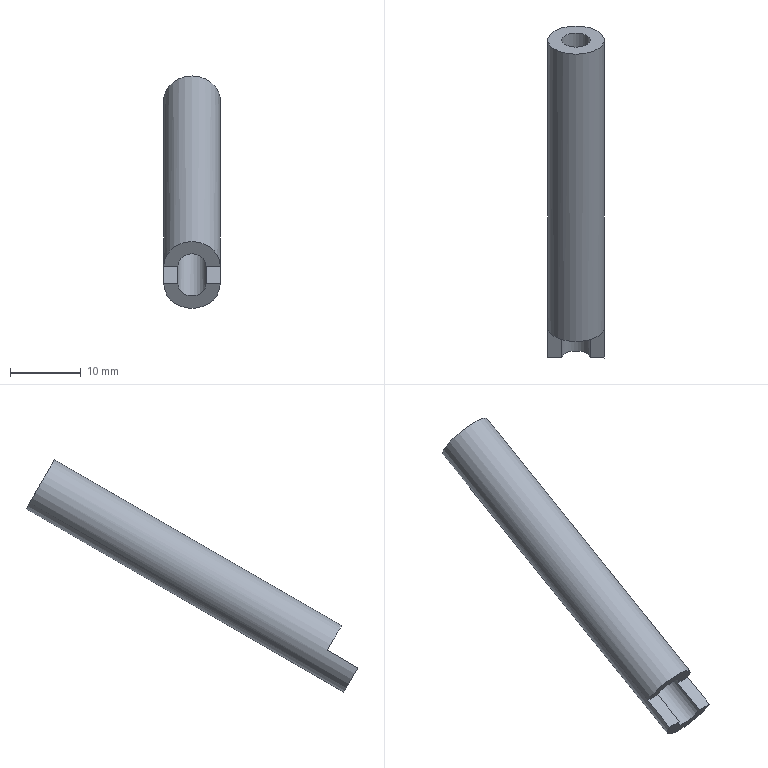Part | NX | features solid 2 | 1 solid | 7 faces | box 8 x 46.958 x 32.885 mm | volume 1862 mm3 | plane 5 | cylinder 2 | commonest cylinder face diameters 4.003 x1 8 x1
STEP:
#1=CARTESIAN_POINT('',(-144.025,135.478,18.602));
#2=VERTEX_POINT('',#1);
#3=CARTESIAN_POINT('',(-136.025,135.478,18.602));
#4=VERTEX_POINT('',#3);
#5=CARTESIAN_POINT('',(-140.025,135.478,18.602));
#6=DIRECTION('',(0.000000832,0.866,0.5));
#7=DIRECTION('',(-1.,0.,0.000001664));
#8=AXIS2_PLACEMENT_3D('',#5,#6,#7);
#9=CIRCLE('',#8,4.);
#10=EDGE_CURVE('',#2,#4,#9,.F.);
#11=ORIENTED_EDGE('',*,*,#10,.T.);
#12=CARTESIAN_POINT('',(-138.023,135.478,18.602));
#13=VERTEX_POINT('',#12);
#14=CARTESIAN_POINT('',(-145.025,135.478,18.602));
#15=DIRECTION('',(1.,0.,-0.000001664));
#16=VECTOR('',#15,1000.);
#17=LINE('',#14,#16);
#18=EDGE_CURVE('',#4,#13,#17,.F.);
#19=ORIENTED_EDGE('',*,*,#18,.T.);
#20=CARTESIAN_POINT('',(-142.026,135.478,18.602));
#21=VERTEX_POINT('',#20);
#22=CARTESIAN_POINT('',(-140.025,135.478,18.602));
#23=DIRECTION('',(0.000000832,0.866,0.5));
#24=DIRECTION('',(-1.,0.,0.000001664));
#25=AXIS2_PLACEMENT_3D('',#22,#23,#24);
#26=CIRCLE('',#25,2.002);
#27=EDGE_CURVE('',#21,#13,#26,.F.);
#28=ORIENTED_EDGE('',*,*,#27,.F.);
#29=CARTESIAN_POINT('',(-145.025,135.478,18.602));
#30=DIRECTION('',(1.,0.,-0.000001664));
#31=VECTOR('',#30,1000.);
#32=LINE('',#29,#31);
#33=EDGE_CURVE('',#21,#2,#32,.F.);
#34=ORIENTED_EDGE('',*,*,#33,.T.);
#35=EDGE_LOOP('',(#11,#19,#28,#34));
#36=FACE_BOUND('',#35,.T.);
#37=CARTESIAN_POINT('',(-140.025,135.478,18.602));
#38=DIRECTION('',(-0.000000832,-0.866,-0.5));
#39=DIRECTION('',(0.,0.5,-0.866));
#40=AXIS2_PLACEMENT_3D('',#37,#38,#39);
#41=PLANE('',#40);
#42=ADVANCED_FACE('',(#36),#41,.T.);
#43=ORIENTED_EDGE('',*,*,#10,.F.);
#44=CARTESIAN_POINT('',(-144.025,139.808,21.102));
#45=VERTEX_POINT('',#44);
#46=CARTESIAN_POINT('',(-144.025,135.478,18.602));
#47=DIRECTION('',(0.000000832,0.866,0.5));
#48=VECTOR('',#47,1000.);
#49=LINE('',#46,#48);
#50=EDGE_CURVE('',#2,#45,#49,.T.);
#51=ORIENTED_EDGE('',*,*,#50,.T.);
#52=CARTESIAN_POINT('',(-136.025,139.808,21.102));
#53=VERTEX_POINT('',#52);
#54=CARTESIAN_POINT('',(-140.025,139.808,21.102));
#55=DIRECTION('',(0.000000832,0.866,0.5));
#56=DIRECTION('',(0.,0.5,-0.866));
#57=AXIS2_PLACEMENT_3D('',#54,#55,#56);
#58=CIRCLE('',#57,4.);
#59=EDGE_CURVE('',#53,#45,#58,.F.);
#60=ORIENTED_EDGE('',*,*,#59,.F.);
#61=CARTESIAN_POINT('',(-136.025,135.478,18.602));
#62=DIRECTION('',(0.000000832,0.866,0.5));
#63=VECTOR('',#62,1000.);
#64=LINE('',#61,#63);
#65=EDGE_CURVE('',#53,#4,#64,.F.);
#66=ORIENTED_EDGE('',*,*,#65,.T.);
#67=EDGE_LOOP('',(#43,#51,#60,#66));
#68=FACE_BOUND('',#67,.T.);
#69=CARTESIAN_POINT('',(-140.025,178.436,48.023));
#70=VERTEX_POINT('',#69);
#71=CARTESIAN_POINT('',(-140.025,180.436,44.559));
#72=DIRECTION('',(-0.000000832,-0.866,-0.5));
#73=DIRECTION('',(0.,-0.5,0.866));
#74=AXIS2_PLACEMENT_3D('',#71,#72,#73);
#75=CIRCLE('',#74,4.);
#76=EDGE_CURVE('',#70,#70,#75,.T.);
#77=ORIENTED_EDGE('',*,*,#76,.T.);
#78=EDGE_LOOP('',(#77));
#79=FACE_BOUND('',#78,.T.);
#80=CARTESIAN_POINT('',(-140.025,135.478,18.602));
#81=DIRECTION('',(0.000000832,0.866,0.5));
#82=DIRECTION('',(0.,-0.5,0.866));
#83=AXIS2_PLACEMENT_3D('',#80,#81,#82);
#84=CYLINDRICAL_SURFACE('',#83,4.);
#85=ADVANCED_FACE('',(#68,#79),#84,.T.);
#86=CARTESIAN_POINT('',(-140.025,179.435,46.293));
#87=VERTEX_POINT('',#86);
#88=CARTESIAN_POINT('',(-140.025,180.436,44.559));
#89=DIRECTION('',(-0.000000832,-0.866,-0.5));
#90=DIRECTION('',(0.,-0.5,0.866));
#91=AXIS2_PLACEMENT_3D('',#88,#89,#90);
#92=CIRCLE('',#91,2.002);
#93=EDGE_CURVE('',#87,#87,#92,.T.);
#94=ORIENTED_EDGE('',*,*,#93,.T.);
#95=EDGE_LOOP('',(#94));
#96=FACE_BOUND('',#95,.T.);
#97=ORIENTED_EDGE('',*,*,#76,.F.);
#98=EDGE_LOOP('',(#97));
#99=FACE_BOUND('',#98,.T.);
#100=CARTESIAN_POINT('',(-150.099,180.935,43.695));
#101=DIRECTION('',(-0.000000832,-0.866,-0.5));
#102=DIRECTION('',(0.000001441,-0.5,0.866));
#103=AXIS2_PLACEMENT_3D('',#100,#101,#102);
#104=PLANE('',#103);
#105=ADVANCED_FACE('',(#96,#99),#104,.F.);
#106=CARTESIAN_POINT('',(-138.023,139.808,21.102));
#107=VERTEX_POINT('',#106);
#108=CARTESIAN_POINT('',(-138.023,135.478,18.602));
#109=DIRECTION('',(0.000000832,0.866,0.5));
#110=VECTOR('',#109,1000.);
#111=LINE('',#108,#110);
#112=EDGE_CURVE('',#107,#13,#111,.F.);
#113=ORIENTED_EDGE('',*,*,#112,.F.);
#114=CARTESIAN_POINT('',(-142.026,139.808,21.102));
#115=VERTEX_POINT('',#114);
#116=CARTESIAN_POINT('',(-140.025,139.808,21.102));
#117=DIRECTION('',(0.000000832,0.866,0.5));
#118=DIRECTION('',(0.,0.5,-0.866));
#119=AXIS2_PLACEMENT_3D('',#116,#117,#118);
#120=CIRCLE('',#119,2.002);
#121=EDGE_CURVE('',#107,#115,#120,.F.);
#122=ORIENTED_EDGE('',*,*,#121,.T.);
#123=CARTESIAN_POINT('',(-142.026,135.478,18.602));
#124=DIRECTION('',(0.000000832,0.866,0.5));
#125=VECTOR('',#124,1000.);
#126=LINE('',#123,#125);
#127=EDGE_CURVE('',#21,#115,#126,.T.);
#128=ORIENTED_EDGE('',*,*,#127,.F.);
#129=ORIENTED_EDGE('',*,*,#27,.T.);
#130=EDGE_LOOP('',(#113,#122,#128,#129));
#131=FACE_BOUND('',#130,.T.);
#132=ORIENTED_EDGE('',*,*,#93,.F.);
#133=EDGE_LOOP('',(#132));
#134=FACE_BOUND('',#133,.T.);
#135=CARTESIAN_POINT('',(-140.025,135.478,18.602));
#136=DIRECTION('',(0.000000832,0.866,0.5));
#137=DIRECTION('',(0.,-0.5,0.866));
#138=AXIS2_PLACEMENT_3D('',#135,#136,#137);
#139=CYLINDRICAL_SURFACE('',#138,2.002);
#140=ADVANCED_FACE('',(#131,#134),#139,.F.);
#141=ORIENTED_EDGE('',*,*,#18,.F.);
#142=ORIENTED_EDGE('',*,*,#65,.F.);
#143=CARTESIAN_POINT('',(-145.025,139.808,21.102));
#144=DIRECTION('',(1.,0.,-0.000001664));
#145=VECTOR('',#144,1000.);
#146=LINE('',#143,#145);
#147=EDGE_CURVE('',#107,#53,#146,.T.);
#148=ORIENTED_EDGE('',*,*,#147,.F.);
#149=ORIENTED_EDGE('',*,*,#112,.T.);
#150=EDGE_LOOP('',(#141,#142,#148,#149));
#151=FACE_BOUND('',#150,.T.);
#152=CARTESIAN_POINT('',(-145.025,135.478,18.602));
#153=DIRECTION('',(-0.000001441,0.5,-0.866));
#154=DIRECTION('',(0.000001665,0.866,0.5));
#155=AXIS2_PLACEMENT_3D('',#152,#153,#154);
#156=PLANE('',#155);
#157=ADVANCED_FACE('',(#151),#156,.F.);
#158=CARTESIAN_POINT('',(-145.025,139.808,21.102));
#159=DIRECTION('',(1.,0.,-0.000001664));
#160=VECTOR('',#159,1000.);
#161=LINE('',#158,#160);
#162=EDGE_CURVE('',#45,#115,#161,.T.);
#163=ORIENTED_EDGE('',*,*,#162,.F.);
#164=ORIENTED_EDGE('',*,*,#50,.F.);
#165=ORIENTED_EDGE('',*,*,#33,.F.);
#166=ORIENTED_EDGE('',*,*,#127,.T.);
#167=EDGE_LOOP('',(#163,#164,#165,#166));
#168=FACE_BOUND('',#167,.T.);
#169=CARTESIAN_POINT('',(-145.025,135.478,18.602));
#170=DIRECTION('',(-0.000001441,0.5,-0.866));
#171=DIRECTION('',(0.000001665,0.866,0.5));
#172=AXIS2_PLACEMENT_3D('',#169,#170,#171);
#173=PLANE('',#172);
#174=ADVANCED_FACE('',(#168),#173,.F.);
#175=ORIENTED_EDGE('',*,*,#59,.T.);
#176=ORIENTED_EDGE('',*,*,#162,.T.);
#177=ORIENTED_EDGE('',*,*,#121,.F.);
#178=ORIENTED_EDGE('',*,*,#147,.T.);
#179=EDGE_LOOP('',(#175,#176,#177,#178));
#180=FACE_BOUND('',#179,.T.);
#181=CARTESIAN_POINT('',(-140.025,139.808,21.102));
#182=DIRECTION('',(-0.000000832,-0.866,-0.5));
#183=DIRECTION('',(0.,0.5,-0.866));
#184=AXIS2_PLACEMENT_3D('',#181,#182,#183);
#185=PLANE('',#184);
#186=ADVANCED_FACE('',(#180),#185,.T.);
#187=CLOSED_SHELL('',(#42,#85,#105,#140,#157,#174,#186));
#188=MANIFOLD_SOLID_BREP('',#187);
#189=(LENGTH_UNIT()NAMED_UNIT(*)SI_UNIT(.MILLI.,.METRE.));
#190=UNCERTAINTY_MEASURE_WITH_UNIT(LENGTH_MEASURE(0.00001),#189,'','');
#191=(NAMED_UNIT(*)PLANE_ANGLE_UNIT()SI_UNIT($,.RADIAN.));
#192=(NAMED_UNIT(*)SI_UNIT($,.STERADIAN.)SOLID_ANGLE_UNIT());
#193=(GEOMETRIC_REPRESENTATION_CONTEXT(3)GLOBAL_UNCERTAINTY_ASSIGNED_CONTEXT((#190))GLOBAL_UNIT_ASSIGNED_CONTEXT((#189,#191,#192))REPRESENTATION_CONTEXT('',''));
#194=ADVANCED_BREP_SHAPE_REPRESENTATION('',(#188),#193);